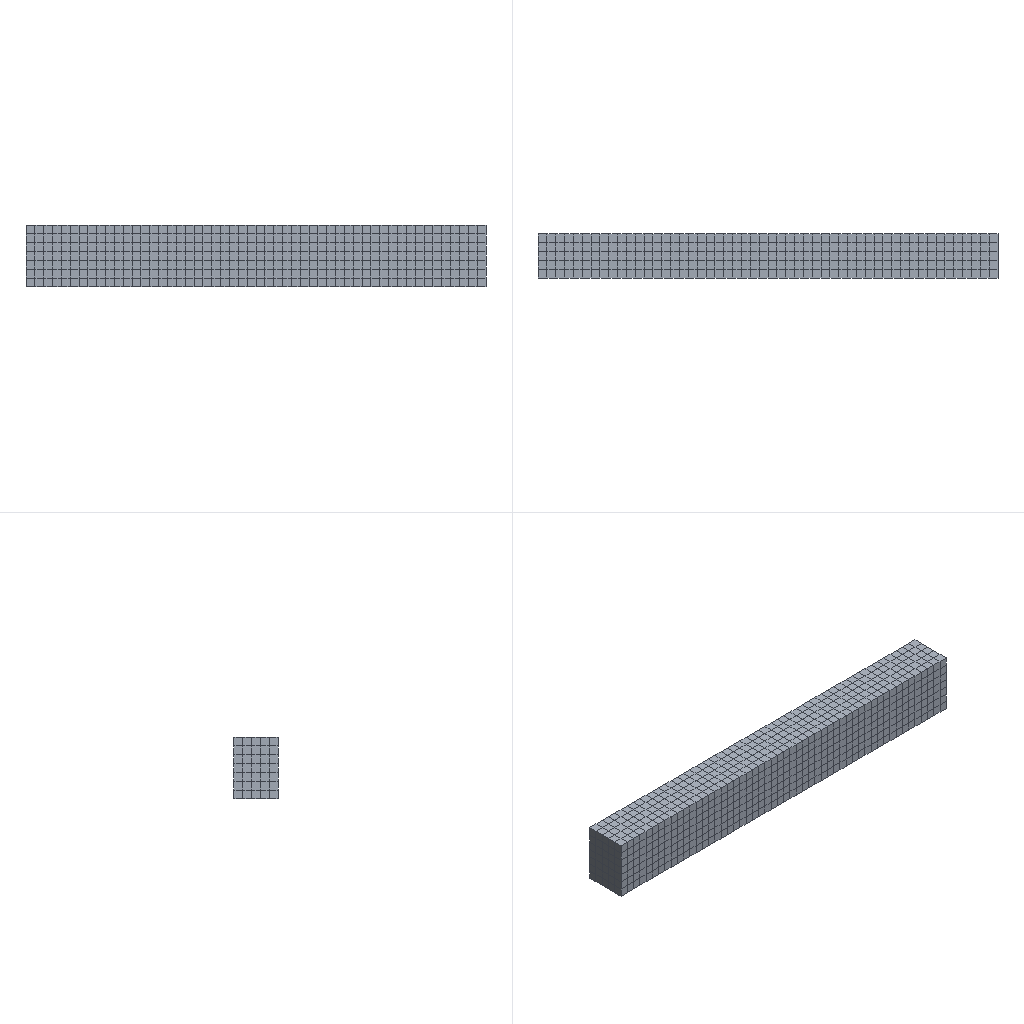Simulation study | abaqus
Set-up summary:
category,name,step,type,value,unit,region
solver,abaqus
solver,version,,,Abaqus/Standard 2020
units,not stated in the deck,,not stated
analysis,deck,,static,static
load_step,Step-1,Step-1,static
load_step,requested,,,1
mesh,nodes,,,8172
mesh,elements,,,7441
element_type,R3D3,,rigid,12
element_type,R3D4,,rigid,4347
element_type,T3D2,,truss,1262
element_type,C3D8R,,solid,1820
load,load commands in deck,,count,1
bc,support commands in deck,,count,7
material,C50,,in results
material,STEEL,,in results
check,setup vs results,,match,"per instance, exact: element labels, types and connectivity; labels of the nodes the elements use; coordinates of those nodes at SINGLE_PRECISION in 55 of 55 instance(s)"
Abaqus input file, long lists of numbers shortened:
*Heading
** Job name: Job-1 Model name: Model-1
** Generated by: Abaqus/CAE 2020
*Preprint, echo=NO, model=NO, history=NO, contact=NO
**
** PARTS
**
*Part, name=concrete
*Node
      1,           0.,        -250.,         350.
      2,           0.,        -200.,         350.
** (2542 more lines like these left out)
*Element, type=C3D8R
   1,   49,   50,   56,   55,    1,    2,    8,    7
   2,   50,   51,   57,   56,    2,    3,    9,    8
** (1818 more lines like these left out)
*Nset, nset=Set-2, generate
    1,  2544,     1
*Elset, elset=Set-2, generate
    1,  1820,     1
** Section: con
*Solid Section, elset=Set-2, material=c50
,
*End Part
**
*Part, name=dan-jin
*Node
      1,       -1840.,           0.,           0.
      2,       -1586.,           0.,           0.
** (9 more lines like these left out)
*Element, type=T3D2
 1,  1,  2
 2,  2,  3
** (8 more lines like these left out)
*Nset, nset=Set-1, generate
  1,  11,   1
*Elset, elset=Set-1, generate
  1,  10,   1
** Section: dan-fi10
*Solid Section, elset=Set-1, material=steel
78.5,
*End Part
**
*Part, name=dan-jin-fi14
*Node
      1,       -1840.,           0.,           0.
      2,       -1586.,           0.,           0.
** (9 more lines like these left out)
*Element, type=T3D2
 1,  1,  2
 2,  2,  3
** (8 more lines like these left out)
*Nset, nset=Set-1, generate
  1,  11,   1
*Elset, elset=Set-1, generate
  1,  10,   1
*Nset, nset=Set-2, generate
  1,  11,   1
*Elset, elset=Set-2, generate
  1,  10,   1
** Section: dan-fi14
*Solid Section, elset=Set-2, material=steel
153.86,
*End Part
**
*Part, name=jin
*Node
      1,         190.,           0.,           0.
      2,         190.,        -290.,           0.
** (24 more lines like these left out)
*Element, type=T3D2
1,  2,  5
2,  5,  6
** (24 more lines like these left out)
*Nset, nset=Set-1, generate
  1,  26,   1
*Elset, elset=Set-1, generate
  1,  26,   1
** Section: Section-1
*Solid Section, elset=Set-1, material=steel
78.5,
*End Part
**
*Part, name=zhicheng
*Node
      1,   10.29,  -17.15,         350.
      2,   10.29,  -17.15,           0.
** (1451 more lines like these left out)
*Element, type=R3D4
   1,    1,    3,   45,   66
   2,    3,    4,   46,   45
** (1447 more lines like these left out)
*Element, type=R3D3
1343, 1393, 1373, 1383
1344, 1386, 1400, 1372
** (2 more lines like these left out)
*Node
   1454,           0.,           0.,         175.
*Nset, nset=zhicheng-RefPt_, internal
1454,
*Elset, elset=zhicheng, generate
    1,  1453,     1
*End Part
**
**
** ASSEMBLY
**
*Assembly, name=Assembly
**
*Instance, name=concrete-1, part=concrete
*End Instance
**
*Instance, name=dan-jin-1, part=dan-jin
       1870.,         -30.,         320.
*End Instance
**
*Instance, name=dan-jin-fi14-1, part=dan-jin-fi14
       1870.,         -30.,          30.
*End Instance
**
*Instance, name=dan-jin-fi14-2, part=dan-jin-fi14
       1870.,        -220.,          30.
*End Instance
**
*Instance, name=dan-jin-2, part=dan-jin
       1870.,        -220.,         320.
*End Instance
**
*Instance, name=jin-1-lin-2-1, part=jin
         60.,         -30.,         320.
         60.,         -30.,         320., 60.577, -30.577, 319.423,         120.
*End Instance
**
*Instance, name=jin-1-lin-3-1, part=jin
         90.,         -30.,         320.
         90.,         -30.,         320., 90.577, -30.577, 319.423,         120.
*End Instance
**
*Instance, name=jin-1-lin-4-1, part=jin
        120.,         -30.,         320.
        120.,         -30.,         320., 120.577, -30.577, 319.423,         120.
*End Instance
**
*Instance, name=jin-1-lin-5-1, part=jin
        150.,         -30.,         320.
        150.,         -30.,         320., 150.577, -30.577, 319.423,         120.
*End Instance
**
*Instance, name=jin-1-lin-6-1, part=jin
        180.,         -30.,         320.
        180.,         -30.,         320., 180.577, -30.577, 319.423,         120.
*End Instance
**
*Instance, name=jin-1-lin-6-1-lin-2-1, part=jin
        240.,         -30.,         320.
        240.,         -30.,         320., 240.577, -30.577, 319.423,         120.
*End Instance
**
*Instance, name=jin-1-lin-6-1-lin-3-1, part=jin
        300.,         -30.,         320.
        300.,         -30.,         320., 300.577, -30.577, 319.423,         120.
*End Instance
**
*Instance, name=jin-1-lin-6-1-lin-4-1, part=jin
        360.,         -30.,         320.
        360.,         -30.,         320., 360.577, -30.577, 319.423,         120.
*End Instance
**
*Instance, name=jin-1-lin-6-1-lin-5-1, part=jin
        420.,         -30.,         320.
        420.,         -30.,         320., 420.577, -30.577, 319.423,         120.
*End Instance
**
*Instance, name=jin-1-lin-6-1-lin-6-1, part=jin
        480.,         -30.,         320.
        480.,         -30.,         320., 480.577, -30.577, 319.423,         120.
*End Instance
**
*Instance, name=jin-1-lin-6-1-lin-7-1, part=jin
        540.,         -30.,         320.
        540.,         -30.,         320., 540.577, -30.577, 319.423,         120.
*End Instance
**
*Instance, name=jin-1-lin-6-1-lin-8-1, part=jin
        600.,         -30.,         320.
        600.,         -30.,         320., 600.577, -30.577, 319.423,         120.
*End Instance
**
*Instance, name=jin-1-lin-6-1-lin-9-1, part=jin
        660.,         -30.,         320.
        660.,         -30.,         320., 660.577, -30.577, 319.423,         120.
*End Instance
**
*Instance, name=jin-1-lin-6-1-lin-10-1, part=jin
        720.,         -30.,         320.
        720.,         -30.,         320., 720.577, -30.577, 319.423,         120.
*End Instance
**
*Instance, name=jin-1-lin-6-1-lin-11-1, part=jin
        780.,         -30.,         320.
        780.,         -30.,         320., 780.577, -30.577, 319.423,         120.
*End Instance
**
*Instance, name=jin-1-lin-6-1-lin-12-1, part=jin
        840.,         -30.,         320.
        840.,         -30.,         320., 840.577, -30.577, 319.423,         120.
*End Instance
**
*Instance, name=jin-1-lin-6-1-lin-13-1, part=jin
        900.,         -30.,         320.
        900.,         -30.,         320., 900.577, -30.577, 319.423,         120.
*End Instance
**
*Instance, name=jin-1-lin-6-1-lin-14-1, part=jin
        960.,         -30.,         320.
        960.,         -30.,         320., 960.577, -30.577, 319.423,         120.
*End Instance
**
*Instance, name=jin-1-lin-6-1-lin-15-1, part=jin
       1020.,         -30.,         320.
       1020.,         -30.,         320., 1020.577, -30.577, 319.423,         120.
*End Instance
**
*Instance, name=jin-1-lin-6-1-lin-16-1, part=jin
       1080.,         -30.,         320.
       1080.,         -30.,         320., 1080.577, -30.577, 319.423,         120.
*End Instance
**
*Instance, name=jin-1-lin-6-1-lin-17-1, part=jin
       1140.,         -30.,         320.
       1140.,         -30.,         320., 1140.577, -30.577, 319.423,         120.
*End Instance
**
*Instance, name=jin-1-lin-6-1-lin-18-1, part=jin
       1200.,         -30.,         320.
       1200.,         -30.,         320., 1200.577, -30.577, 319.423,         120.
*End Instance
**
*Instance, name=jin-1-lin-6-1-lin-19-1, part=jin
       1260.,         -30.,         320.
       1260.,         -30.,         320., 1260.577, -30.577, 319.423,         120.
*End Instance
**
*Instance, name=jin-1-lin-6-1-lin-20-1, part=jin
       1320.,         -30.,         320.
       1320.,         -30.,         320., 1320.577, -30.577, 319.423,         120.
*End Instance
**
*Instance, name=jin-1-lin-6-1-lin-21-1, part=jin
       1380.,         -30.,         320.
       1380.,         -30.,         320., 1380.577, -30.577, 319.423,         120.
*End Instance
**
*Instance, name=jin-1-lin-6-1-lin-22-1, part=jin
       1440.,         -30.,         320.
       1440.,         -30.,         320., 1440.577, -30.577, 319.423,         120.
*End Instance
**
*Instance, name=jin-1-lin-6-1-lin-23-1, part=jin
       1500.,         -30.,         320.
       1500.,         -30.,         320., 1500.577, -30.577, 319.423,         120.
*End Instance
**
*Instance, name=jin-1-lin-6-1-lin-24-1, part=jin
       1560.,         -30.,         320.
       1560.,         -30.,         320., 1560.577, -30.577, 319.423,         120.
*End Instance
**
*Instance, name=jin-1-lin-6-1-lin-25-1, part=jin
       1620.,         -30.,         320.
       1620.,         -30.,         320., 1620.577, -30.577, 319.423,         120.
*End Instance
**
*Instance, name=jin-1-lin-6-1-lin-26-1, part=jin
       1680.,         -30.,         320.
       1680.,         -30.,         320., 1680.577, -30.577, 319.423,         120.
*End Instance
**
*Instance, name=jin-1-lin-6-1-lin-27-1, part=jin
       1740.,         -30.,         320.
       1740.,         -30.,         320., 1740.577, -30.577, 319.423,         120.
*End Instance
**
*Instance, name=jin-1-lin-6-1-lin-28-1, part=jin
       1800.,         -30.,         320.
       1800.,         -30.,         320., 1800.577, -30.577, 319.423,         120.
*End Instance
**
*Instance, name=jin-1-lin-6-1-lin-29-1, part=jin
       1860.,         -30.,         320.
       1860.,         -30.,         320., 1860.577, -30.577, 319.423,         120.
*End Instance
**
*Instance, name=jin-1-lin-6-1-lin-30-1, part=jin
       1920.,         -30.,         320.
       1920.,         -30.,         320., 1920.577, -30.577, 319.423,         120.
*End Instance
**
*Instance, name=jin-1-lin-6-1-lin-31-1, part=jin
       1980.,         -30.,         320.
       1980.,         -30.,         320., 1980.577, -30.577, 319.423,         120.
*End Instance
**
*Instance, name=jin-1-lin-6-1-lin-32-1, part=jin
       2040.,         -30.,         320.
       2040.,         -30.,         320., 2040.577, -30.577, 319.423,         120.
*End Instance
**
*Instance, name=jin-1-lin-6-1-lin-33-1, part=jin
       2100.,         -30.,         320.
       2100.,         -30.,         320., 2100.577, -30.577, 319.423,         120.
*End Instance
**
*Instance, name=jin-1-lin-6-1-lin-34-1, part=jin
       2160.,         -30.,         320.
       2160.,         -30.,         320., 2160.577, -30.577, 319.423,         120.
*End Instance
**
*Instance, name=jin-1-lin-6-1-lin-35-1, part=jin
       2220.,         -30.,         320.
       2220.,         -30.,         320., 2220.577, -30.577, 319.423,         120.
*End Instance
**
*Instance, name=jin-1-lin-6-1-lin-36-1, part=jin
       2280.,         -30.,         320.
       2280.,         -30.,         320., 2280.577, -30.577, 319.423,         120.
*End Instance
**
*Instance, name=jin-1-lin-6-1-lin-37-1, part=jin
       2340.,         -30.,         320.
       2340.,         -30.,         320., 2340.577, -30.577, 319.423,         120.
*End Instance
**
*Instance, name=jin-1-lin-6-1-lin-38-1, part=jin
       2400.,         -30.,         320.
       2400.,         -30.,         320., 2400.577, -30.577, 319.423,         120.
*End Instance
**
*Instance, name=jin-1-lin-6-1-lin-38-1-lin-2-1, part=jin
       2430.,         -30.,         320.
       2430.,         -30.,         320., 2430.577, -30.577, 319.423,         120.
*End Instance
**
*Instance, name=jin-1-lin-6-1-lin-38-1-lin-3-1, part=jin
       2460.,         -30.,         320.
       2460.,         -30.,         320., 2460.577, -30.577, 319.423,         120.
*End Instance
**
*Instance, name=jin-1-lin-6-1-lin-38-1-lin-4-1, part=jin
       2490.,         -30.,         320.
       2490.,         -30.,         320., 2490.577, -30.577, 319.423,         120.
*End Instance
**
*Instance, name=jin-1-lin-6-1-lin-38-1-lin-5-1, part=jin
       2520.,         -30.,         320.
       2520.,         -30.,         320., 2520.577, -30.577, 319.423,         120.
*End Instance
**
*Instance, name=jin-1-lin-6-1-lin-38-1-lin-6-1, part=jin
       2550.,         -30.,         320.
       2550.,         -30.,         320., 2550.577, -30.577, 319.423,         120.
*End Instance
**
*Instance, name=zhicheng-1, part=zhicheng
        150.,          55.,         -20.
        150.,          55.,         -20., 151.,          55.,         -20., 90.
*End Instance
**
*Instance, name=zhicheng-1-lin-2-1, part=zhicheng
       2450.,          55.,         -20.
       2450.,          55.,         -20., 2451.,          55.,         -20., 90.
*End Instance
**
*Instance, name=zhicheng-2, part=zhicheng
       1300.,          50.,         370.
       1300.,          50.,         370., 1301.,          50.,         370., 90.
*End Instance
**
*Nset, nset=Set-1, instance=zhicheng-1
 1454,
*Nset, nset=Set-1, instance=zhicheng-1-lin-2-1
 1454,
*Nset, nset=Set-4, instance=zhicheng-2
 1454,
*Nset, nset=m_Set-2, instance=dan-jin-1, generate
  1,  11,   1
*Nset, nset=m_Set-2, instance=dan-jin-fi14-1, generate
  1,  11,   1
*Nset, nset=m_Set-2, instance=dan-jin-2, generate
  1,  11,   1
*Nset, nset=m_Set-2, instance=jin-1-lin-3-1, generate
  1,  26,   1
*Nset, nset=m_Set-2, instance=jin-1-lin-6-1-lin-6-1, generate
  1,  26,   1
*Nset, nset=m_Set-2, instance=jin-1-lin-6-1-lin-22-1, generate
  1,  26,   1
*Nset, nset=m_Set-2, instance=jin-1-lin-6-1-lin-38-1, generate
  1,  26,   1
*Nset, nset=m_Set-2, instance=jin-1-lin-6-1-lin-14-1, generate
  1,  26,   1
*Nset, nset=m_Set-2, instance=jin-1-lin-6-1-lin-30-1, generate
  1,  26,   1
*Nset, nset=m_Set-2, instance=jin-1-lin-6-1-lin-2-1, generate
  1,  26,   1
*Nset, nset=m_Set-2, instance=jin-1-lin-6-1-lin-10-1, generate
  1,  26,   1
*Nset, nset=m_Set-2, instance=jin-1-lin-6-1-lin-26-1, generate
  1,  26,   1
*Nset, nset=m_Set-2, instance=jin-1-lin-6-1-lin-38-1-lin-5-1, generate
  1,  26,   1
*Nset, nset=m_Set-2, instance=jin-1-lin-6-1-lin-18-1, generate
  1,  26,   1
*Nset, nset=m_Set-2, instance=jin-1-lin-6-1-lin-34-1, generate
  1,  26,   1
*Nset, nset=m_Set-2, instance=jin-1-lin-5-1, generate
  1,  26,   1
*Nset, nset=m_Set-2, instance=jin-1-lin-6-1-lin-8-1, generate
  1,  26,   1
*Nset, nset=m_Set-2, instance=jin-1-lin-6-1-lin-24-1, generate
  1,  26,   1
*Nset, nset=m_Set-2, instance=jin-1-lin-6-1-lin-38-1-lin-3-1, generate
  1,  26,   1
*Nset, nset=m_Set-2, instance=jin-1-lin-6-1-lin-16-1, generate
  1,  26,   1
*Nset, nset=m_Set-2, instance=jin-1-lin-6-1-lin-32-1, generate
  1,  26,   1
*Nset, nset=m_Set-2, instance=jin-1-lin-6-1-lin-4-1, generate
  1,  26,   1
*Nset, nset=m_Set-2, instance=jin-1-lin-6-1-lin-12-1, generate
  1,  26,   1
*Nset, nset=m_Set-2, instance=jin-1-lin-6-1-lin-28-1, generate
  1,  26,   1
*Nset, nset=m_Set-2, instance=jin-1-lin-6-1-lin-20-1, generate
  1,  26,   1
*Nset, nset=m_Set-2, instance=jin-1-lin-6-1-lin-36-1, generate
  1,  26,   1
*Nset, nset=m_Set-2, instance=dan-jin-fi14-2, generate
  1,  11,   1
*Nset, nset=m_Set-2, instance=jin-1-lin-4-1, generate
  1,  26,   1
*Nset, nset=m_Set-2, instance=jin-1-lin-6-1-lin-7-1, generate
  1,  26,   1
*Nset, nset=m_Set-2, instance=jin-1-lin-6-1-lin-23-1, generate
  1,  26,   1
*Nset, nset=m_Set-2, instance=jin-1-lin-6-1-lin-38-1-lin-2-1, generate
  1,  26,   1
*Nset, nset=m_Set-2, instance=jin-1-lin-6-1-lin-15-1, generate
  1,  26,   1
*Nset, nset=m_Set-2, instance=jin-1-lin-6-1-lin-31-1, generate
  1,  26,   1
*Nset, nset=m_Set-2, instance=jin-1-lin-6-1-lin-3-1, generate
  1,  26,   1
*Nset, nset=m_Set-2, instance=jin-1-lin-6-1-lin-11-1, generate
  1,  26,   1
*Nset, nset=m_Set-2, instance=jin-1-lin-6-1-lin-27-1, generate
  1,  26,   1
*Nset, nset=m_Set-2, instance=jin-1-lin-6-1-lin-38-1-lin-6-1, generate
  1,  26,   1
*Nset, nset=m_Set-2, instance=jin-1-lin-6-1-lin-19-1, generate
  1,  26,   1
*Nset, nset=m_Set-2, instance=jin-1-lin-6-1-lin-35-1, generate
  1,  26,   1
*Nset, nset=m_Set-2, instance=jin-1-lin-2-1, generate
  1,  26,   1
*Nset, nset=m_Set-2, instance=jin-1-lin-6-1, generate
  1,  26,   1
*Nset, nset=m_Set-2, instance=jin-1-lin-6-1-lin-9-1, generate
  1,  26,   1
*Nset, nset=m_Set-2, instance=jin-1-lin-6-1-lin-25-1, generate
  1,  26,   1
*Nset, nset=m_Set-2, instance=jin-1-lin-6-1-lin-38-1-lin-4-1, generate
  1,  26,   1
*Nset, nset=m_Set-2, instance=jin-1-lin-6-1-lin-17-1, generate
  1,  26,   1
*Nset, nset=m_Set-2, instance=jin-1-lin-6-1-lin-33-1, generate
  1,  26,   1
*Nset, nset=m_Set-2, instance=jin-1-lin-6-1-lin-5-1, generate
  1,  26,   1
*Nset, nset=m_Set-2, instance=jin-1-lin-6-1-lin-13-1, generate
  1,  26,   1
*Nset, nset=m_Set-2, instance=jin-1-lin-6-1-lin-29-1, generate
  1,  26,   1
*Nset, nset=m_Set-2, instance=jin-1-lin-6-1-lin-21-1, generate
  1,  26,   1
*Nset, nset=m_Set-2, instance=jin-1-lin-6-1-lin-37-1, generate
  1,  26,   1
*Elset, elset=m_Set-2, instance=dan-jin-1, generate
  1,  10,   1
*Elset, elset=m_Set-2, instance=dan-jin-fi14-1, generate
  1,  10,   1
*Elset, elset=m_Set-2, instance=dan-jin-2, generate
  1,  10,   1
*Elset, elset=m_Set-2, instance=jin-1-lin-3-1, generate
  1,  26,   1
*Elset, elset=m_Set-2, instance=jin-1-lin-6-1-lin-6-1, generate
  1,  26,   1
*Elset, elset=m_Set-2, instance=jin-1-lin-6-1-lin-22-1, generate
  1,  26,   1
*Elset, elset=m_Set-2, instance=jin-1-lin-6-1-lin-38-1, generate
  1,  26,   1
*Elset, elset=m_Set-2, instance=jin-1-lin-6-1-lin-14-1, generate
  1,  26,   1
*Elset, elset=m_Set-2, instance=jin-1-lin-6-1-lin-30-1, generate
  1,  26,   1
*Elset, elset=m_Set-2, instance=jin-1-lin-6-1-lin-2-1, generate
  1,  26,   1
*Elset, elset=m_Set-2, instance=jin-1-lin-6-1-lin-10-1, generate
  1,  26,   1
*Elset, elset=m_Set-2, instance=jin-1-lin-6-1-lin-26-1, generate
  1,  26,   1
*Elset, elset=m_Set-2, instance=jin-1-lin-6-1-lin-38-1-lin-5-1, generate
  1,  26,   1
*Elset, elset=m_Set-2, instance=jin-1-lin-6-1-lin-18-1, generate
  1,  26,   1
*Elset, elset=m_Set-2, instance=jin-1-lin-6-1-lin-34-1, generate
  1,  26,   1
*Elset, elset=m_Set-2, instance=jin-1-lin-5-1, generate
  1,  26,   1
*Elset, elset=m_Set-2, instance=jin-1-lin-6-1-lin-8-1, generate
  1,  26,   1
*Elset, elset=m_Set-2, instance=jin-1-lin-6-1-lin-24-1, generate
  1,  26,   1
*Elset, elset=m_Set-2, instance=jin-1-lin-6-1-lin-38-1-lin-3-1, generate
  1,  26,   1
*Elset, elset=m_Set-2, instance=jin-1-lin-6-1-lin-16-1, generate
  1,  26,   1
*Elset, elset=m_Set-2, instance=jin-1-lin-6-1-lin-32-1, generate
  1,  26,   1
*Elset, elset=m_Set-2, instance=jin-1-lin-6-1-lin-4-1, generate
  1,  26,   1
*Elset, elset=m_Set-2, instance=jin-1-lin-6-1-lin-12-1, generate
  1,  26,   1
*Elset, elset=m_Set-2, instance=jin-1-lin-6-1-lin-28-1, generate
  1,  26,   1
*Elset, elset=m_Set-2, instance=jin-1-lin-6-1-lin-20-1, generate
  1,  26,   1
*Elset, elset=m_Set-2, instance=jin-1-lin-6-1-lin-36-1, generate
  1,  26,   1
*Elset, elset=m_Set-2, instance=dan-jin-fi14-2, generate
  1,  10,   1
*Elset, elset=m_Set-2, instance=jin-1-lin-4-1, generate
  1,  26,   1
*Elset, elset=m_Set-2, instance=jin-1-lin-6-1-lin-7-1, generate
  1,  26,   1
*Elset, elset=m_Set-2, instance=jin-1-lin-6-1-lin-23-1, generate
  1,  26,   1
*Elset, elset=m_Set-2, instance=jin-1-lin-6-1-lin-38-1-lin-2-1, generate
  1,  26,   1
*Elset, elset=m_Set-2, instance=jin-1-lin-6-1-lin-15-1, generate
  1,  26,   1
*Elset, elset=m_Set-2, instance=jin-1-lin-6-1-lin-31-1, generate
  1,  26,   1
*Elset, elset=m_Set-2, instance=jin-1-lin-6-1-lin-3-1, generate
  1,  26,   1
*Elset, elset=m_Set-2, instance=jin-1-lin-6-1-lin-11-1, generate
  1,  26,   1
*Elset, elset=m_Set-2, instance=jin-1-lin-6-1-lin-27-1, generate
  1,  26,   1
*Elset, elset=m_Set-2, instance=jin-1-lin-6-1-lin-38-1-lin-6-1, generate
  1,  26,   1
*Elset, elset=m_Set-2, instance=jin-1-lin-6-1-lin-19-1, generate
  1,  26,   1
*Elset, elset=m_Set-2, instance=jin-1-lin-6-1-lin-35-1, generate
  1,  26,   1
*Elset, elset=m_Set-2, instance=jin-1-lin-2-1, generate
  1,  26,   1
*Elset, elset=m_Set-2, instance=jin-1-lin-6-1, generate
  1,  26,   1
*Elset, elset=m_Set-2, instance=jin-1-lin-6-1-lin-9-1, generate
  1,  26,   1
*Elset, elset=m_Set-2, instance=jin-1-lin-6-1-lin-25-1, generate
  1,  26,   1
*Elset, elset=m_Set-2, instance=jin-1-lin-6-1-lin-38-1-lin-4-1, generate
  1,  26,   1
*Elset, elset=m_Set-2, instance=jin-1-lin-6-1-lin-17-1, generate
  1,  26,   1
*Elset, elset=m_Set-2, instance=jin-1-lin-6-1-lin-33-1, generate
  1,  26,   1
*Elset, elset=m_Set-2, instance=jin-1-lin-6-1-lin-5-1, generate
  1,  26,   1
*Elset, elset=m_Set-2, instance=jin-1-lin-6-1-lin-13-1, generate
  1,  26,   1
*Elset, elset=m_Set-2, instance=jin-1-lin-6-1-lin-29-1, generate
  1,  26,   1
*Elset, elset=m_Set-2, instance=jin-1-lin-6-1-lin-21-1, generate
  1,  26,   1
*Elset, elset=m_Set-2, instance=jin-1-lin-6-1-lin-37-1, generate
  1,  26,   1
*Nset, nset=s_Set-2, instance=concrete-1, generate
    1,  2544,     1
*Elset, elset=s_Set-2, instance=concrete-1, generate
    1,  1820,     1
*Rigid Body, ref node=zhicheng-1.zhicheng-RefPt_, elset=zhicheng-1.zhicheng
*Rigid Body, ref node=zhicheng-1-lin-2-1.zhicheng-RefPt_, elset=zhicheng-1-lin-2-1.zhicheng
*Rigid Body, ref node=zhicheng-2.zhicheng-RefPt_, elset=zhicheng-2.zhicheng
** Constraint: Constraint-1
*Embedded Element, host elset=s_Set-2
m_Set-2
*Elset, elset=__Int-1_gcs0_7_SPOS, internal, instance=zhicheng-1, generate
    1,  1342,     1
*Surface, type=ELEMENT, name=_Int-1_gcs0_7, internal
__Int-1_gcs0_7_SPOS, SPOS
*Elset, elset=__Int-1_gcs0_10_SNEG, internal, instance=zhicheng-1, generate
    1,  1342,     1
*Surface, type=ELEMENT, name=_Int-1_gcs0_10, internal
__Int-1_gcs0_10_SNEG, SNEG
*Elset, elset=__Int-1_gcs0_13_SPOS, internal, instance=zhicheng-1-lin-2-1, generate
    1,  1342,     1
*Surface, type=ELEMENT, name=_Int-1_gcs0_13, internal
__Int-1_gcs0_13_SPOS, SPOS
*Elset, elset=__Int-1_gcs0_16_SNEG, internal, instance=zhicheng-1-lin-2-1, generate
    1,  1342,     1
*Surface, type=ELEMENT, name=_Int-1_gcs0_16, internal
__Int-1_gcs0_16_SNEG, SNEG
*Elset, elset=__Int-1_gcs0_19_SPOS, internal, instance=zhicheng-2, generate
    1,  1342,     1
*Surface, type=ELEMENT, name=_Int-1_gcs0_19, internal
__Int-1_gcs0_19_SPOS, SPOS
*Elset, elset=__Int-1_gcs0_22_SNEG, internal, instance=zhicheng-2, generate
    1,  1342,     1
*Surface, type=ELEMENT, name=_Int-1_gcs0_22, internal
__Int-1_gcs0_22_SNEG, SNEG
*End Assembly
*Amplitude, name=Amp-1
             0.,              0.,             10.,              1.
**
** MATERIALS
**
*Material, name=c50
*Density
 2.5e-09,
*Elastic
35000., 0.2
*Concrete Damaged Plasticity
30.,    0.1,   1.16, 0.6667,   0.05
*Concrete Compression Hardening
 15.4,      0.
 16.9,  0.0002
 19.6, 0.00048
 20.1, 0.00079
  20., 0.00095
 19.6,  0.0011
 19.1, 0.00127
 18.6, 0.00143
 17.9,  0.0016
 17.2, 0.00177
 16.6, 0.00194
 15.9, 0.00211
 15.3, 0.00228
 14.7, 0.00245
 14.1, 0.00261
 13.5, 0.00278
  13., 0.00294
 12.5,  0.0031
  12., 0.00327
 11.6, 0.00343
 11.2, 0.00359
 10.8, 0.00375
 10.4, 0.00391
 10.1, 0.00406
*Concrete Tension Stiffening
 2.06,      0.
 1.92,   2e-05
 1.72,   4e-05
 1.53,   6e-05
 1.37,   8e-05
 1.24,  0.0001
 1.13, 0.00011
 1.04, 0.00013
 0.97, 0.00015
  0.9, 0.00016
 0.85, 0.00018
*Concrete Compression Damage
     0.,      0.
 0.0841,   9e-05
 0.0933,  0.0001
 0.1091, 0.00013
 0.1418,  0.0002
 0.2407, 0.00048
  0.322, 0.00079
 0.3557, 0.00095
 0.3886,  0.0011
 0.4201, 0.00127
 0.4499, 0.00143
 0.4778,  0.0016
 0.5039, 0.00177
 0.5282, 0.00194
 0.5506, 0.00211
 0.5715, 0.00228
 0.5908, 0.00245
 0.6086, 0.00261
 0.6252, 0.00278
 0.6406, 0.00294
 0.6549,  0.0031
 0.6682, 0.00327
 0.6806, 0.00343
 0.6922, 0.00359
  0.703, 0.00375
 0.7131, 0.00391
 0.7227, 0.00406
   0.74, 0.00438
 0.7554, 0.00469
 0.7691,   0.005
 0.7815, 0.00531
 0.7926, 0.00561
 0.8026, 0.00592
 0.8118, 0.00622
 0.8202, 0.00653
 0.8278, 0.00683
 0.8349, 0.00713
*Concrete Tension Damage
      0.,      0.
 0.1181,   2e-05
 0.2281,   4e-05
 0.3187,   6e-05
 0.3919,   8e-05
 0.4512,  0.0001
 0.5, 0.00011
  0.5407, 0.00013
 0.575, 0.00015
 0.6043, 0.00016
 0.6297, 0.00018
 0.7177, 0.00025
 0.7702, 0.00033
 0.8053,  0.0004
 0.8304, 0.00047
 0.8494, 0.00054
  0.8643, 0.00061
 0.8763, 0.00068
 0.8862, 0.00075
*Material, name=steel
*Density
 7.8e-09,
*Elastic
210000., 0.3
*Plastic
235.,0.
**
** INTERACTION PROPERTIES
**
*Surface Interaction, name=IntProp-1
1.,
*Friction, slip tolerance=0.005
 0.4,
*Surface Behavior, pressure-overclosure=HARD
**
** INTERACTIONS
**
** Interaction: Int-1
*Contact
*Contact Inclusions, ALL EXTERIOR
*Contact Property Assignment
 ,  , IntProp-1
*Surface Property Assignment, property=GEOMETRIC CORRECTION
_Int-1_gcs0_7, Circumferential, 150., 55., -20.,  150., 54., -20.
_Int-1_gcs0_10, Circumferential, 150., 55., -20.,  150., 54., -20.
_Int-1_gcs0_13, Circumferential, 2450., 55., -20.,  2450., 54., -20.
_Int-1_gcs0_16, Circumferential, 2450., 55., -20.,  2450., 54., -20.
_Int-1_gcs0_19, Circumferential, 1300., 50., 370.,  1300., 49., 370.
_Int-1_gcs0_22, Circumferential, 1300., 50., 370.,  1300., 49., 370.
** ----------------------------------------------------------------
**
** STEP: Step-1
**
*Step, name=Step-1, nlgeom=YES, inc=10000
*Static, stabilize=0.0002, allsdtol=0.05, continue=NO
0.1, 10., 0.0001, 10.
**
** BOUNDARY CONDITIONS
**
** Name: BC-1 Type: 对称/反对称/完全固定
*Boundary
Set-1, ENCASTRE
** Name: BC-2 Type: 位移/转角
*Boundary
Set-4, 1, 1
Set-4, 2, 2
Set-4, 3, 3, -150.
Set-4, 4, 4
Set-4, 5, 5
Set-4, 6, 6
**
** OUTPUT REQUESTS
**
*Restart, write, frequency=0
**
** FIELD OUTPUT: F-Output-1
**
*Output, field
*Node Output
CF, RF, U
*Element Output, directions=YES
DAMAGEC, DAMAGET, LE, PE, PEEQ, PEMAG, S, SDEG
*Contact Output
CDISP, CSTRESS
**
** HISTORY OUTPUT: H-Output-1
**
*Output, history
*Node Output, nset=Set-4
RF3, RM3, U3
*End Step
Results summary:
result,step,,completed,increments=181 time=10.0/10.0
result,analysis,,,static
result,last_loadstep,,,1
result,primary field,,,U
result,reaction total,,FX,-12.584,model units
result,reaction total,,FY,0.01488,model units
result,reaction total,,FZ,-596.754,model units